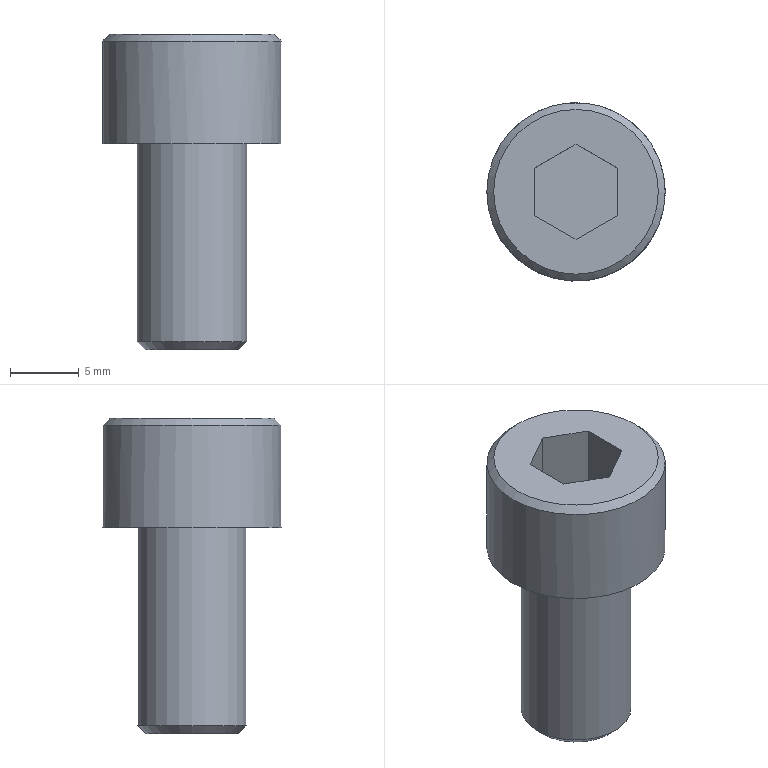Part | STEP file | gslz 2016.10.28-6_id122_x_t | 1 solid | 14 faces | box 13 x 13 x 23 mm | volume 1651 mm3 | plane 10 | cylinder 2 | cone 2 | commonest cylinder face diameters 8 x1 13 x1
STEP:
#1=CARTESIAN_POINT('',(-79.,21.,10.));
#2=VERTEX_POINT('',#1);
#3=CARTESIAN_POINT('',(-85.,21.,10.));
#4=DIRECTION('',(0.,0.,1.));
#5=DIRECTION('',(1.,0.,0.));
#6=AXIS2_PLACEMENT_3D('',#3,#4,#5);
#7=CIRCLE('',#6,6.);
#8=EDGE_CURVE('',#2,#2,#7,.T.);
#9=ORIENTED_EDGE('',*,*,#8,.T.);
#10=EDGE_LOOP('',(#9));
#11=FACE_BOUND('',#10,.T.);
#12=CARTESIAN_POINT('',(-88.,22.732,10.));
#13=VERTEX_POINT('',#12);
#14=CARTESIAN_POINT('',(-88.,19.268,10.));
#15=VERTEX_POINT('',#14);
#16=CARTESIAN_POINT('',(-88.,22.732,10.));
#17=DIRECTION('',(0.,-1.,0.));
#18=VECTOR('',#17,1.);
#19=LINE('',#16,#18);
#20=EDGE_CURVE('',#13,#15,#19,.T.);
#21=ORIENTED_EDGE('',*,*,#20,.F.);
#22=CARTESIAN_POINT('',(-85.,24.464,10.));
#23=VERTEX_POINT('',#22);
#24=CARTESIAN_POINT('',(-85.,24.464,10.));
#25=DIRECTION('',(-0.866,-0.5,0.));
#26=VECTOR('',#25,1.);
#27=LINE('',#24,#26);
#28=EDGE_CURVE('',#23,#13,#27,.T.);
#29=ORIENTED_EDGE('',*,*,#28,.F.);
#30=CARTESIAN_POINT('',(-82.,22.732,10.));
#31=VERTEX_POINT('',#30);
#32=CARTESIAN_POINT('',(-82.,22.732,10.));
#33=DIRECTION('',(-0.866,0.5,0.));
#34=VECTOR('',#33,1.);
#35=LINE('',#32,#34);
#36=EDGE_CURVE('',#31,#23,#35,.T.);
#37=ORIENTED_EDGE('',*,*,#36,.F.);
#38=CARTESIAN_POINT('',(-82.,19.268,10.));
#39=VERTEX_POINT('',#38);
#40=CARTESIAN_POINT('',(-82.,19.268,10.));
#41=DIRECTION('',(0.,1.,0.));
#42=VECTOR('',#41,1.);
#43=LINE('',#40,#42);
#44=EDGE_CURVE('',#39,#31,#43,.T.);
#45=ORIENTED_EDGE('',*,*,#44,.F.);
#46=CARTESIAN_POINT('',(-85.,17.536,10.));
#47=VERTEX_POINT('',#46);
#48=CARTESIAN_POINT('',(-85.,17.536,10.));
#49=DIRECTION('',(0.866,0.5,0.));
#50=VECTOR('',#49,1.);
#51=LINE('',#48,#50);
#52=EDGE_CURVE('',#47,#39,#51,.T.);
#53=ORIENTED_EDGE('',*,*,#52,.F.);
#54=CARTESIAN_POINT('',(-88.,19.268,10.));
#55=DIRECTION('',(0.866,-0.5,0.));
#56=VECTOR('',#55,1.);
#57=LINE('',#54,#56);
#58=EDGE_CURVE('',#15,#47,#57,.T.);
#59=ORIENTED_EDGE('',*,*,#58,.F.);
#60=EDGE_LOOP('',(#21,#29,#37,#45,#53,#59));
#61=FACE_BOUND('',#60,.T.);
#62=CARTESIAN_POINT('',(-85.,21.,10.));
#63=DIRECTION('',(0.,0.,1.));
#64=DIRECTION('',(-1.,0.,0.));
#65=AXIS2_PLACEMENT_3D('',#62,#63,#64);
#66=PLANE('',#65);
#67=ADVANCED_FACE('',(#11,#61),#66,.T.);
#68=CARTESIAN_POINT('',(-88.4,21.,-13.));
#69=VERTEX_POINT('',#68);
#70=CARTESIAN_POINT('',(-85.,21.,-13.));
#71=DIRECTION('',(0.,0.,-1.));
#72=DIRECTION('',(-1.,0.,0.));
#73=AXIS2_PLACEMENT_3D('',#70,#71,#72);
#74=CIRCLE('',#73,3.4);
#75=EDGE_CURVE('',#69,#69,#74,.T.);
#76=ORIENTED_EDGE('',*,*,#75,.T.);
#77=EDGE_LOOP('',(#76));
#78=FACE_OUTER_BOUND('',#77,.T.);
#79=CARTESIAN_POINT('',(-85.,21.,-13.));
#80=DIRECTION('',(0.,0.,-1.));
#81=DIRECTION('',(1.,0.,0.));
#82=AXIS2_PLACEMENT_3D('',#79,#80,#81);
#83=PLANE('',#82);
#84=ADVANCED_FACE('',(#78),#83,.T.);
#85=CARTESIAN_POINT('',(-89.,21.,-12.4));
#86=VERTEX_POINT('',#85);
#87=CARTESIAN_POINT('',(-85.,21.,-12.4));
#88=DIRECTION('',(0.,0.,1.));
#89=DIRECTION('',(-1.,0.,0.));
#90=AXIS2_PLACEMENT_3D('',#87,#88,#89);
#91=CIRCLE('',#90,4.);
#92=EDGE_CURVE('',#86,#86,#91,.T.);
#93=ORIENTED_EDGE('',*,*,#92,.T.);
#94=EDGE_LOOP('',(#93));
#95=FACE_BOUND('',#94,.T.);
#96=CARTESIAN_POINT('',(-89.,21.,2.));
#97=VERTEX_POINT('',#96);
#98=CARTESIAN_POINT('',(-85.,21.,2.));
#99=DIRECTION('',(0.,0.,-1.));
#100=DIRECTION('',(-1.,0.,0.));
#101=AXIS2_PLACEMENT_3D('',#98,#99,#100);
#102=CIRCLE('',#101,4.);
#103=EDGE_CURVE('',#97,#97,#102,.T.);
#104=ORIENTED_EDGE('',*,*,#103,.T.);
#105=EDGE_LOOP('',(#104));
#106=FACE_BOUND('',#105,.T.);
#107=CARTESIAN_POINT('',(-85.,21.,0.));
#108=DIRECTION('',(0.,0.,-1.));
#109=DIRECTION('',(-1.,0.,0.));
#110=AXIS2_PLACEMENT_3D('',#107,#108,#109);
#111=CYLINDRICAL_SURFACE('',#110,4.);
#112=ADVANCED_FACE('',(#95,#106),#111,.T.);
#113=ORIENTED_EDGE('',*,*,#103,.F.);
#114=EDGE_LOOP('',(#113));
#115=FACE_BOUND('',#114,.T.);
#116=CARTESIAN_POINT('',(-91.5,21.,2.));
#117=VERTEX_POINT('',#116);
#118=CARTESIAN_POINT('',(-85.,21.,2.));
#119=DIRECTION('',(0.,0.,-1.));
#120=DIRECTION('',(-1.,0.,0.));
#121=AXIS2_PLACEMENT_3D('',#118,#119,#120);
#122=CIRCLE('',#121,6.5);
#123=EDGE_CURVE('',#117,#117,#122,.T.);
#124=ORIENTED_EDGE('',*,*,#123,.T.);
#125=EDGE_LOOP('',(#124));
#126=FACE_BOUND('',#125,.T.);
#127=CARTESIAN_POINT('',(-85.,21.,2.));
#128=DIRECTION('',(0.,0.,-1.));
#129=DIRECTION('',(1.,0.,0.));
#130=AXIS2_PLACEMENT_3D('',#127,#128,#129);
#131=PLANE('',#130);
#132=ADVANCED_FACE('',(#115,#126),#131,.T.);
#133=CARTESIAN_POINT('',(-78.5,21.,9.5));
#134=VERTEX_POINT('',#133);
#135=CARTESIAN_POINT('',(-85.,21.,9.5));
#136=DIRECTION('',(0.,0.,-1.));
#137=DIRECTION('',(1.,0.,0.));
#138=AXIS2_PLACEMENT_3D('',#135,#136,#137);
#139=CIRCLE('',#138,6.5);
#140=EDGE_CURVE('',#134,#134,#139,.T.);
#141=ORIENTED_EDGE('',*,*,#140,.T.);
#142=EDGE_LOOP('',(#141));
#143=FACE_BOUND('',#142,.T.);
#144=ORIENTED_EDGE('',*,*,#123,.F.);
#145=EDGE_LOOP('',(#144));
#146=FACE_BOUND('',#145,.T.);
#147=CARTESIAN_POINT('',(-85.,21.,13.));
#148=DIRECTION('',(0.,0.,-1.));
#149=DIRECTION('',(-1.,0.,0.));
#150=AXIS2_PLACEMENT_3D('',#147,#148,#149);
#151=CYLINDRICAL_SURFACE('',#150,6.5);
#152=ADVANCED_FACE('',(#143,#146),#151,.T.);
#153=ORIENTED_EDGE('',*,*,#92,.F.);
#154=EDGE_LOOP('',(#153));
#155=FACE_BOUND('',#154,.T.);
#156=ORIENTED_EDGE('',*,*,#75,.F.);
#157=EDGE_LOOP('',(#156));
#158=FACE_BOUND('',#157,.T.);
#159=CARTESIAN_POINT('',(-85.,21.,-13.));
#160=DIRECTION('',(0.,0.,1.));
#161=DIRECTION('',(1.,0.,0.));
#162=AXIS2_PLACEMENT_3D('',#159,#160,#161);
#163=CONICAL_SURFACE('',#162,3.4,45.);
#164=ADVANCED_FACE('',(#155,#158),#163,.T.);
#165=ORIENTED_EDGE('',*,*,#20,.T.);
#166=CARTESIAN_POINT('',(-88.,19.268,5.));
#167=VERTEX_POINT('',#166);
#168=CARTESIAN_POINT('',(-88.,19.268,5.));
#169=DIRECTION('',(0.,0.,-1.));
#170=VECTOR('',#169,1.);
#171=LINE('',#168,#170);
#172=EDGE_CURVE('',#15,#167,#171,.T.);
#173=ORIENTED_EDGE('',*,*,#172,.T.);
#174=CARTESIAN_POINT('',(-88.,22.732,5.));
#175=VERTEX_POINT('',#174);
#176=CARTESIAN_POINT('',(-88.,22.732,5.));
#177=DIRECTION('',(0.,1.,0.));
#178=VECTOR('',#177,1.);
#179=LINE('',#176,#178);
#180=EDGE_CURVE('',#167,#175,#179,.T.);
#181=ORIENTED_EDGE('',*,*,#180,.T.);
#182=CARTESIAN_POINT('',(-88.,22.732,5.));
#183=DIRECTION('',(0.,0.,-1.));
#184=VECTOR('',#183,1.);
#185=LINE('',#182,#184);
#186=EDGE_CURVE('',#13,#175,#185,.T.);
#187=ORIENTED_EDGE('',*,*,#186,.F.);
#188=EDGE_LOOP('',(#165,#173,#181,#187));
#189=FACE_OUTER_BOUND('',#188,.T.);
#190=CARTESIAN_POINT('',(-88.,22.732,5.));
#191=DIRECTION('',(-1.,0.,0.));
#192=DIRECTION('',(0.,0.,1.));
#193=AXIS2_PLACEMENT_3D('',#190,#191,#192);
#194=PLANE('',#193);
#195=ADVANCED_FACE('',(#189),#194,.F.);
#196=ORIENTED_EDGE('',*,*,#58,.T.);
#197=CARTESIAN_POINT('',(-85.,17.536,5.));
#198=VERTEX_POINT('',#197);
#199=CARTESIAN_POINT('',(-85.,17.536,5.));
#200=DIRECTION('',(0.,0.,-1.));
#201=VECTOR('',#200,1.);
#202=LINE('',#199,#201);
#203=EDGE_CURVE('',#47,#198,#202,.T.);
#204=ORIENTED_EDGE('',*,*,#203,.T.);
#205=CARTESIAN_POINT('',(-88.,19.268,5.));
#206=DIRECTION('',(-0.866,0.5,0.));
#207=VECTOR('',#206,1.);
#208=LINE('',#205,#207);
#209=EDGE_CURVE('',#198,#167,#208,.T.);
#210=ORIENTED_EDGE('',*,*,#209,.T.);
#211=ORIENTED_EDGE('',*,*,#172,.F.);
#212=EDGE_LOOP('',(#196,#204,#210,#211));
#213=FACE_OUTER_BOUND('',#212,.T.);
#214=CARTESIAN_POINT('',(-88.,19.268,5.));
#215=DIRECTION('',(-0.5,-0.866,0.));
#216=DIRECTION('',(-0.866,0.5,0.));
#217=AXIS2_PLACEMENT_3D('',#214,#215,#216);
#218=PLANE('',#217);
#219=ADVANCED_FACE('',(#213),#218,.F.);
#220=ORIENTED_EDGE('',*,*,#52,.T.);
#221=CARTESIAN_POINT('',(-82.,19.268,5.));
#222=VERTEX_POINT('',#221);
#223=CARTESIAN_POINT('',(-82.,19.268,5.));
#224=DIRECTION('',(0.,0.,-1.));
#225=VECTOR('',#224,1.);
#226=LINE('',#223,#225);
#227=EDGE_CURVE('',#39,#222,#226,.T.);
#228=ORIENTED_EDGE('',*,*,#227,.T.);
#229=CARTESIAN_POINT('',(-85.,17.536,5.));
#230=DIRECTION('',(-0.866,-0.5,0.));
#231=VECTOR('',#230,1.);
#232=LINE('',#229,#231);
#233=EDGE_CURVE('',#222,#198,#232,.T.);
#234=ORIENTED_EDGE('',*,*,#233,.T.);
#235=ORIENTED_EDGE('',*,*,#203,.F.);
#236=EDGE_LOOP('',(#220,#228,#234,#235));
#237=FACE_OUTER_BOUND('',#236,.T.);
#238=CARTESIAN_POINT('',(-85.,17.536,5.));
#239=DIRECTION('',(0.5,-0.866,0.));
#240=DIRECTION('',(-0.866,-0.5,0.));
#241=AXIS2_PLACEMENT_3D('',#238,#239,#240);
#242=PLANE('',#241);
#243=ADVANCED_FACE('',(#237),#242,.F.);
#244=ORIENTED_EDGE('',*,*,#44,.T.);
#245=CARTESIAN_POINT('',(-82.,22.732,5.));
#246=VERTEX_POINT('',#245);
#247=CARTESIAN_POINT('',(-82.,22.732,5.));
#248=DIRECTION('',(0.,0.,-1.));
#249=VECTOR('',#248,1.);
#250=LINE('',#247,#249);
#251=EDGE_CURVE('',#31,#246,#250,.T.);
#252=ORIENTED_EDGE('',*,*,#251,.T.);
#253=CARTESIAN_POINT('',(-82.,19.268,5.));
#254=DIRECTION('',(0.,-1.,0.));
#255=VECTOR('',#254,1.);
#256=LINE('',#253,#255);
#257=EDGE_CURVE('',#246,#222,#256,.T.);
#258=ORIENTED_EDGE('',*,*,#257,.T.);
#259=ORIENTED_EDGE('',*,*,#227,.F.);
#260=EDGE_LOOP('',(#244,#252,#258,#259));
#261=FACE_OUTER_BOUND('',#260,.T.);
#262=CARTESIAN_POINT('',(-82.,19.268,5.));
#263=DIRECTION('',(1.,0.,0.));
#264=DIRECTION('',(0.,0.,1.));
#265=AXIS2_PLACEMENT_3D('',#262,#263,#264);
#266=PLANE('',#265);
#267=ADVANCED_FACE('',(#261),#266,.F.);
#268=ORIENTED_EDGE('',*,*,#36,.T.);
#269=CARTESIAN_POINT('',(-85.,24.464,5.));
#270=VERTEX_POINT('',#269);
#271=CARTESIAN_POINT('',(-85.,24.464,5.));
#272=DIRECTION('',(0.,0.,-1.));
#273=VECTOR('',#272,1.);
#274=LINE('',#271,#273);
#275=EDGE_CURVE('',#23,#270,#274,.T.);
#276=ORIENTED_EDGE('',*,*,#275,.T.);
#277=CARTESIAN_POINT('',(-82.,22.732,5.));
#278=DIRECTION('',(0.866,-0.5,0.));
#279=VECTOR('',#278,1.);
#280=LINE('',#277,#279);
#281=EDGE_CURVE('',#270,#246,#280,.T.);
#282=ORIENTED_EDGE('',*,*,#281,.T.);
#283=ORIENTED_EDGE('',*,*,#251,.F.);
#284=EDGE_LOOP('',(#268,#276,#282,#283));
#285=FACE_OUTER_BOUND('',#284,.T.);
#286=CARTESIAN_POINT('',(-82.,22.732,5.));
#287=DIRECTION('',(0.5,0.866,0.));
#288=DIRECTION('',(0.866,-0.5,0.));
#289=AXIS2_PLACEMENT_3D('',#286,#287,#288);
#290=PLANE('',#289);
#291=ADVANCED_FACE('',(#285),#290,.F.);
#292=ORIENTED_EDGE('',*,*,#28,.T.);
#293=ORIENTED_EDGE('',*,*,#186,.T.);
#294=CARTESIAN_POINT('',(-85.,24.464,5.));
#295=DIRECTION('',(0.866,0.5,0.));
#296=VECTOR('',#295,1.);
#297=LINE('',#294,#296);
#298=EDGE_CURVE('',#175,#270,#297,.T.);
#299=ORIENTED_EDGE('',*,*,#298,.T.);
#300=ORIENTED_EDGE('',*,*,#275,.F.);
#301=EDGE_LOOP('',(#292,#293,#299,#300));
#302=FACE_OUTER_BOUND('',#301,.T.);
#303=CARTESIAN_POINT('',(-85.,24.464,5.));
#304=DIRECTION('',(-0.5,0.866,0.));
#305=DIRECTION('',(0.866,0.5,0.));
#306=AXIS2_PLACEMENT_3D('',#303,#304,#305);
#307=PLANE('',#306);
#308=ADVANCED_FACE('',(#302),#307,.F.);
#309=ORIENTED_EDGE('',*,*,#180,.F.);
#310=ORIENTED_EDGE('',*,*,#209,.F.);
#311=ORIENTED_EDGE('',*,*,#233,.F.);
#312=ORIENTED_EDGE('',*,*,#257,.F.);
#313=ORIENTED_EDGE('',*,*,#281,.F.);
#314=ORIENTED_EDGE('',*,*,#298,.F.);
#315=EDGE_LOOP('',(#309,#310,#311,#312,#313,#314));
#316=FACE_OUTER_BOUND('',#315,.T.);
#317=CARTESIAN_POINT('',(-88.,19.268,5.));
#318=DIRECTION('',(0.,0.,1.));
#319=DIRECTION('',(-1.,0.,0.));
#320=AXIS2_PLACEMENT_3D('',#317,#318,#319);
#321=PLANE('',#320);
#322=ADVANCED_FACE('',(#316),#321,.T.);
#323=ORIENTED_EDGE('',*,*,#8,.F.);
#324=EDGE_LOOP('',(#323));
#325=FACE_BOUND('',#324,.T.);
#326=ORIENTED_EDGE('',*,*,#140,.F.);
#327=EDGE_LOOP('',(#326));
#328=FACE_BOUND('',#327,.T.);
#329=CARTESIAN_POINT('',(-85.,21.,9.5));
#330=DIRECTION('',(0.,0.,-1.));
#331=DIRECTION('',(-1.,0.,0.));
#332=AXIS2_PLACEMENT_3D('',#329,#330,#331);
#333=CONICAL_SURFACE('',#332,6.5,45.);
#334=ADVANCED_FACE('',(#325,#328),#333,.T.);
#335=CLOSED_SHELL('',(#67,#84,#112,#132,#152,#164,#195,#219,#243,#267,#291,#308,#322,#334));
#336=MANIFOLD_SOLID_BREP('',#335);
#337=(LENGTH_UNIT()NAMED_UNIT(*)SI_UNIT(.MILLI.,.METRE.));
#338=UNCERTAINTY_MEASURE_WITH_UNIT(LENGTH_MEASURE(0.00002),#337,'','');
#339=(NAMED_UNIT(*)PLANE_ANGLE_UNIT()SI_UNIT($,.RADIAN.));
#340=PLANE_ANGLE_MEASURE_WITH_UNIT(PLANE_ANGLE_MEASURE(0.01745),#339);
#341=DIMENSIONAL_EXPONENTS(0.,0.,0.,0.,0.,0.,0.);
#342=(CONVERSION_BASED_UNIT('DEGREE',#340)NAMED_UNIT(#341)PLANE_ANGLE_UNIT());
#343=(NAMED_UNIT(*)SI_UNIT($,.STERADIAN.)SOLID_ANGLE_UNIT());
#344=(GEOMETRIC_REPRESENTATION_CONTEXT(3)GLOBAL_UNCERTAINTY_ASSIGNED_CONTEXT((#338))GLOBAL_UNIT_ASSIGNED_CONTEXT((#337,#342,#343))REPRESENTATION_CONTEXT('',''));
#345=ADVANCED_BREP_SHAPE_REPRESENTATION('',(#336),#344);